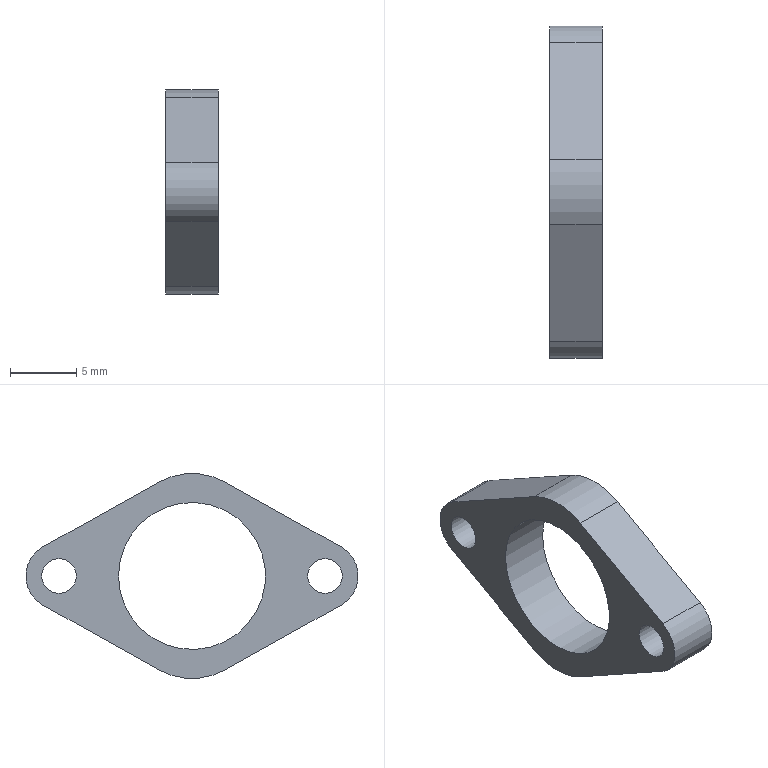Part | STEP file | Dodanie-wyci_gni_cie1_6 | 1 solid | 13 faces | box 3.95 x 25 x 15.427 mm | volume 542.296 mm3 | cylinder 7 | plane 6 | commonest cylinder face diameters 2.6 x2 5 x2 10 x2 11.05 x1
STEP:
#1=CARTESIAN_POINT('',(0.,0.,0.));
#2=DIRECTION('',(0.,0.,1.));
#3=DIRECTION('',(1.,0.,0.));
#4=AXIS2_PLACEMENT_3D('',#1,#2,#3);
#5=CARTESIAN_POINT('',(-64.621,79.561,-75.356));
#6=VERTEX_POINT('',#5);
#7=CARTESIAN_POINT('',(-64.621,78.261,-75.356));
#8=DIRECTION('',(1.,0.,0.));
#9=DIRECTION('',(0.,1.,0.));
#10=AXIS2_PLACEMENT_3D('',#7,#8,#9);
#11=CIRCLE('',#10,1.3);
#12=CARTESIAN_POINT('',(-64.621,78.261,-75.356));
#13=DIRECTION('',(1.,0.,0.));
#14=DIRECTION('',(0.,1.,0.));
#15=AXIS2_PLACEMENT_3D('',#12,#13,#14);
#16=CYLINDRICAL_SURFACE('',#15,1.3);
#17=CARTESIAN_POINT('',(0.,0.));
#18=DIRECTION('',(1.,0.));
#19=VECTOR('',#18,1.);
#20=LINE('',#17,#19);
#21=(GEOMETRIC_REPRESENTATION_CONTEXT(2)PARAMETRIC_REPRESENTATION_CONTEXT()REPRESENTATION_CONTEXT('',''));
#22=DEFINITIONAL_REPRESENTATION('',(#20),#21);
#23=PCURVE('',#16,#22);
#24=CARTESIAN_POINT('',(-64.621,88.261,-75.356));
#25=DIRECTION('',(-1.,0.,0.));
#26=DIRECTION('',(0.,-1.,0.));
#27=AXIS2_PLACEMENT_3D('',#24,#25,#26);
#28=PLANE('',#27);
#29=CARTESIAN_POINT('',(8.7,0.000278));
#30=CARTESIAN_POINT('',(8.7,2.252));
#31=CARTESIAN_POINT('',(10.65,1.126));
#32=CARTESIAN_POINT('',(12.6,0.000278));
#33=CARTESIAN_POINT('',(10.65,-1.126));
#34=CARTESIAN_POINT('',(8.7,-2.251));
#35=CARTESIAN_POINT('',(8.7,0.000278));
#36=(BOUNDED_CURVE()B_SPLINE_CURVE(2,(#29,#30,#31,#32,#33,#34,#35),.UNSPECIFIED.,.T.,.F.)B_SPLINE_CURVE_WITH_KNOTS((1,2,2,2,2,1),(-2.094,0.,2.094,4.189,6.283,8.378),.UNSPECIFIED.)CURVE()GEOMETRIC_REPRESENTATION_ITEM()RATIONAL_B_SPLINE_CURVE((1.,0.5,1.,0.5,1.,0.5,1.))REPRESENTATION_ITEM(''));
#37=(GEOMETRIC_REPRESENTATION_CONTEXT(2)PARAMETRIC_REPRESENTATION_CONTEXT()REPRESENTATION_CONTEXT('',''));
#38=DEFINITIONAL_REPRESENTATION('',(#36),#37);
#39=PCURVE('',#28,#38);
#40=SURFACE_CURVE('',#11,(#23,#39),.PCURVE_S1.);
#41=EDGE_CURVE('',#6,#6,#40,.T.);
#42=ORIENTED_EDGE('',*,*,#41,.T.);
#43=CARTESIAN_POINT('',(-60.671,79.561,-75.356));
#44=VERTEX_POINT('',#43);
#45=CARTESIAN_POINT('',(-60.671,79.561,-75.356));
#46=DIRECTION('',(-1.,0.,0.));
#47=VECTOR('',#46,1.);
#48=LINE('',#45,#47);
#49=CARTESIAN_POINT('',(6.283,3.95));
#50=DIRECTION('',(0.,-1.));
#51=VECTOR('',#50,1.);
#52=LINE('',#49,#51);
#53=(GEOMETRIC_REPRESENTATION_CONTEXT(2)PARAMETRIC_REPRESENTATION_CONTEXT()REPRESENTATION_CONTEXT('',''));
#54=DEFINITIONAL_REPRESENTATION('',(#52),#53);
#55=PCURVE('',#16,#54);
#56=CARTESIAN_POINT('',(0.,3.95));
#57=DIRECTION('',(0.,-1.));
#58=VECTOR('',#57,1.);
#59=LINE('',#56,#58);
#60=(GEOMETRIC_REPRESENTATION_CONTEXT(2)PARAMETRIC_REPRESENTATION_CONTEXT()REPRESENTATION_CONTEXT('',''));
#61=DEFINITIONAL_REPRESENTATION('',(#59),#60);
#62=PCURVE('',#16,#61);
#63=SEAM_CURVE('',#48,(#55,#62),.PCURVE_S1.);
#64=EDGE_CURVE('',#44,#6,#63,.T.);
#65=ORIENTED_EDGE('',*,*,#64,.F.);
#66=CARTESIAN_POINT('',(-60.671,78.261,-75.356));
#67=DIRECTION('',(-1.,0.,0.));
#68=DIRECTION('',(0.,1.,0.));
#69=AXIS2_PLACEMENT_3D('',#66,#67,#68);
#70=CIRCLE('',#69,1.3);
#71=CARTESIAN_POINT('',(6.283,3.95));
#72=DIRECTION('',(-1.,0.));
#73=VECTOR('',#72,1.);
#74=LINE('',#71,#73);
#75=(GEOMETRIC_REPRESENTATION_CONTEXT(2)PARAMETRIC_REPRESENTATION_CONTEXT()REPRESENTATION_CONTEXT('',''));
#76=DEFINITIONAL_REPRESENTATION('',(#74),#75);
#77=PCURVE('',#16,#76);
#78=CARTESIAN_POINT('',(-60.671,88.261,-75.356));
#79=DIRECTION('',(-1.,0.,0.));
#80=DIRECTION('',(0.,-1.,0.));
#81=AXIS2_PLACEMENT_3D('',#78,#79,#80);
#82=PLANE('',#81);
#83=CARTESIAN_POINT('',(10.,0.000278));
#84=DIRECTION('',(-1.,0.));
#85=AXIS2_PLACEMENT_2D('',#83,#84);
#86=CIRCLE('',#85,1.3);
#87=(GEOMETRIC_REPRESENTATION_CONTEXT(2)PARAMETRIC_REPRESENTATION_CONTEXT()REPRESENTATION_CONTEXT('',''));
#88=DEFINITIONAL_REPRESENTATION('',(#86),#87);
#89=PCURVE('',#82,#88);
#90=SURFACE_CURVE('',#70,(#77,#89),.PCURVE_S1.);
#91=EDGE_CURVE('',#44,#44,#90,.T.);
#92=ORIENTED_EDGE('',*,*,#91,.T.);
#93=ORIENTED_EDGE('',*,*,#64,.T.);
#94=EDGE_LOOP('',(#42,#65,#92,#93));
#95=FACE_BOUND('',#94,.F.);
#96=ADVANCED_FACE('',(#95),#16,.F.);
#97=CARTESIAN_POINT('',(-64.621,93.786,-75.356));
#98=VERTEX_POINT('',#97);
#99=CARTESIAN_POINT('',(-64.621,88.261,-75.356));
#100=DIRECTION('',(1.,0.,0.));
#101=DIRECTION('',(0.,1.,0.));
#102=AXIS2_PLACEMENT_3D('',#99,#100,#101);
#103=CIRCLE('',#102,5.525);
#104=CARTESIAN_POINT('',(-64.621,88.261,-75.356));
#105=DIRECTION('',(1.,0.,0.));
#106=DIRECTION('',(0.,1.,0.));
#107=AXIS2_PLACEMENT_3D('',#104,#105,#106);
#108=CYLINDRICAL_SURFACE('',#107,5.525);
#109=CARTESIAN_POINT('',(0.,0.));
#110=DIRECTION('',(1.,0.));
#111=VECTOR('',#110,1.);
#112=LINE('',#109,#111);
#113=(GEOMETRIC_REPRESENTATION_CONTEXT(2)PARAMETRIC_REPRESENTATION_CONTEXT()REPRESENTATION_CONTEXT('',''));
#114=DEFINITIONAL_REPRESENTATION('',(#112),#113);
#115=PCURVE('',#108,#114);
#116=CARTESIAN_POINT('',(-5.525,0.000278));
#117=CARTESIAN_POINT('',(-5.525,9.57));
#118=CARTESIAN_POINT('',(2.763,4.785));
#119=CARTESIAN_POINT('',(11.05,0.000278));
#120=CARTESIAN_POINT('',(2.763,-4.785));
#121=CARTESIAN_POINT('',(-5.525,-9.569));
#122=CARTESIAN_POINT('',(-5.525,0.000278));
#123=(BOUNDED_CURVE()B_SPLINE_CURVE(2,(#116,#117,#118,#119,#120,#121,#122),.UNSPECIFIED.,.T.,.F.)B_SPLINE_CURVE_WITH_KNOTS((1,2,2,2,2,1),(-2.094,0.,2.094,4.189,6.283,8.378),.UNSPECIFIED.)CURVE()GEOMETRIC_REPRESENTATION_ITEM()RATIONAL_B_SPLINE_CURVE((1.,0.5,1.,0.5,1.,0.5,1.))REPRESENTATION_ITEM(''));
#124=(GEOMETRIC_REPRESENTATION_CONTEXT(2)PARAMETRIC_REPRESENTATION_CONTEXT()REPRESENTATION_CONTEXT('',''));
#125=DEFINITIONAL_REPRESENTATION('',(#123),#124);
#126=PCURVE('',#28,#125);
#127=SURFACE_CURVE('',#103,(#115,#126),.PCURVE_S1.);
#128=EDGE_CURVE('',#98,#98,#127,.T.);
#129=ORIENTED_EDGE('',*,*,#128,.T.);
#130=CARTESIAN_POINT('',(-60.671,93.786,-75.356));
#131=VERTEX_POINT('',#130);
#132=CARTESIAN_POINT('',(-60.671,93.786,-75.356));
#133=DIRECTION('',(-1.,0.,0.));
#134=VECTOR('',#133,1.);
#135=LINE('',#132,#134);
#136=CARTESIAN_POINT('',(6.283,3.95));
#137=DIRECTION('',(0.,-1.));
#138=VECTOR('',#137,1.);
#139=LINE('',#136,#138);
#140=(GEOMETRIC_REPRESENTATION_CONTEXT(2)PARAMETRIC_REPRESENTATION_CONTEXT()REPRESENTATION_CONTEXT('',''));
#141=DEFINITIONAL_REPRESENTATION('',(#139),#140);
#142=PCURVE('',#108,#141);
#143=CARTESIAN_POINT('',(0.,3.95));
#144=DIRECTION('',(0.,-1.));
#145=VECTOR('',#144,1.);
#146=LINE('',#143,#145);
#147=(GEOMETRIC_REPRESENTATION_CONTEXT(2)PARAMETRIC_REPRESENTATION_CONTEXT()REPRESENTATION_CONTEXT('',''));
#148=DEFINITIONAL_REPRESENTATION('',(#146),#147);
#149=PCURVE('',#108,#148);
#150=SEAM_CURVE('',#135,(#142,#149),.PCURVE_S1.);
#151=EDGE_CURVE('',#131,#98,#150,.T.);
#152=ORIENTED_EDGE('',*,*,#151,.F.);
#153=CARTESIAN_POINT('',(-60.671,88.261,-75.356));
#154=DIRECTION('',(-1.,0.,0.));
#155=DIRECTION('',(0.,1.,0.));
#156=AXIS2_PLACEMENT_3D('',#153,#154,#155);
#157=CIRCLE('',#156,5.525);
#158=CARTESIAN_POINT('',(6.283,3.95));
#159=DIRECTION('',(-1.,0.));
#160=VECTOR('',#159,1.);
#161=LINE('',#158,#160);
#162=(GEOMETRIC_REPRESENTATION_CONTEXT(2)PARAMETRIC_REPRESENTATION_CONTEXT()REPRESENTATION_CONTEXT('',''));
#163=DEFINITIONAL_REPRESENTATION('',(#161),#162);
#164=PCURVE('',#108,#163);
#165=CARTESIAN_POINT('',(0.,0.000278));
#166=DIRECTION('',(-1.,0.));
#167=AXIS2_PLACEMENT_2D('',#165,#166);
#168=CIRCLE('',#167,5.525);
#169=(GEOMETRIC_REPRESENTATION_CONTEXT(2)PARAMETRIC_REPRESENTATION_CONTEXT()REPRESENTATION_CONTEXT('',''));
#170=DEFINITIONAL_REPRESENTATION('',(#168),#169);
#171=PCURVE('',#82,#170);
#172=SURFACE_CURVE('',#157,(#164,#171),.PCURVE_S1.);
#173=EDGE_CURVE('',#131,#131,#172,.T.);
#174=ORIENTED_EDGE('',*,*,#173,.T.);
#175=ORIENTED_EDGE('',*,*,#151,.T.);
#176=EDGE_LOOP('',(#129,#152,#174,#175));
#177=FACE_BOUND('',#176,.F.);
#178=ADVANCED_FACE('',(#177),#108,.F.);
#179=CARTESIAN_POINT('',(-64.621,99.561,-75.356));
#180=VERTEX_POINT('',#179);
#181=CARTESIAN_POINT('',(-64.621,98.261,-75.356));
#182=DIRECTION('',(1.,0.,0.));
#183=DIRECTION('',(0.,1.,0.));
#184=AXIS2_PLACEMENT_3D('',#181,#182,#183);
#185=CIRCLE('',#184,1.3);
#186=CARTESIAN_POINT('',(-64.621,98.261,-75.356));
#187=DIRECTION('',(1.,0.,0.));
#188=DIRECTION('',(0.,1.,0.));
#189=AXIS2_PLACEMENT_3D('',#186,#187,#188);
#190=CYLINDRICAL_SURFACE('',#189,1.3);
#191=CARTESIAN_POINT('',(0.,0.));
#192=DIRECTION('',(1.,0.));
#193=VECTOR('',#192,1.);
#194=LINE('',#191,#193);
#195=(GEOMETRIC_REPRESENTATION_CONTEXT(2)PARAMETRIC_REPRESENTATION_CONTEXT()REPRESENTATION_CONTEXT('',''));
#196=DEFINITIONAL_REPRESENTATION('',(#194),#195);
#197=PCURVE('',#190,#196);
#198=CARTESIAN_POINT('',(-11.3,0.000278));
#199=CARTESIAN_POINT('',(-11.3,2.252));
#200=CARTESIAN_POINT('',(-9.35,1.126));
#201=CARTESIAN_POINT('',(-7.4,0.000278));
#202=CARTESIAN_POINT('',(-9.35,-1.126));
#203=CARTESIAN_POINT('',(-11.3,-2.251));
#204=CARTESIAN_POINT('',(-11.3,0.000278));
#205=(BOUNDED_CURVE()B_SPLINE_CURVE(2,(#198,#199,#200,#201,#202,#203,#204),.UNSPECIFIED.,.T.,.F.)B_SPLINE_CURVE_WITH_KNOTS((1,2,2,2,2,1),(-2.094,0.,2.094,4.189,6.283,8.378),.UNSPECIFIED.)CURVE()GEOMETRIC_REPRESENTATION_ITEM()RATIONAL_B_SPLINE_CURVE((1.,0.5,1.,0.5,1.,0.5,1.))REPRESENTATION_ITEM(''));
#206=(GEOMETRIC_REPRESENTATION_CONTEXT(2)PARAMETRIC_REPRESENTATION_CONTEXT()REPRESENTATION_CONTEXT('',''));
#207=DEFINITIONAL_REPRESENTATION('',(#205),#206);
#208=PCURVE('',#28,#207);
#209=SURFACE_CURVE('',#185,(#197,#208),.PCURVE_S1.);
#210=EDGE_CURVE('',#180,#180,#209,.T.);
#211=ORIENTED_EDGE('',*,*,#210,.T.);
#212=CARTESIAN_POINT('',(-60.671,99.561,-75.356));
#213=VERTEX_POINT('',#212);
#214=CARTESIAN_POINT('',(-60.671,99.561,-75.356));
#215=DIRECTION('',(-1.,0.,0.));
#216=VECTOR('',#215,1.);
#217=LINE('',#214,#216);
#218=CARTESIAN_POINT('',(6.283,3.95));
#219=DIRECTION('',(0.,-1.));
#220=VECTOR('',#219,1.);
#221=LINE('',#218,#220);
#222=(GEOMETRIC_REPRESENTATION_CONTEXT(2)PARAMETRIC_REPRESENTATION_CONTEXT()REPRESENTATION_CONTEXT('',''));
#223=DEFINITIONAL_REPRESENTATION('',(#221),#222);
#224=PCURVE('',#190,#223);
#225=CARTESIAN_POINT('',(0.,3.95));
#226=DIRECTION('',(0.,-1.));
#227=VECTOR('',#226,1.);
#228=LINE('',#225,#227);
#229=(GEOMETRIC_REPRESENTATION_CONTEXT(2)PARAMETRIC_REPRESENTATION_CONTEXT()REPRESENTATION_CONTEXT('',''));
#230=DEFINITIONAL_REPRESENTATION('',(#228),#229);
#231=PCURVE('',#190,#230);
#232=SEAM_CURVE('',#217,(#224,#231),.PCURVE_S1.);
#233=EDGE_CURVE('',#213,#180,#232,.T.);
#234=ORIENTED_EDGE('',*,*,#233,.F.);
#235=CARTESIAN_POINT('',(-60.671,98.261,-75.356));
#236=DIRECTION('',(-1.,0.,0.));
#237=DIRECTION('',(0.,1.,0.));
#238=AXIS2_PLACEMENT_3D('',#235,#236,#237);
#239=CIRCLE('',#238,1.3);
#240=CARTESIAN_POINT('',(6.283,3.95));
#241=DIRECTION('',(-1.,0.));
#242=VECTOR('',#241,1.);
#243=LINE('',#240,#242);
#244=(GEOMETRIC_REPRESENTATION_CONTEXT(2)PARAMETRIC_REPRESENTATION_CONTEXT()REPRESENTATION_CONTEXT('',''));
#245=DEFINITIONAL_REPRESENTATION('',(#243),#244);
#246=PCURVE('',#190,#245);
#247=CARTESIAN_POINT('',(-10.,0.000278));
#248=DIRECTION('',(-1.,0.));
#249=AXIS2_PLACEMENT_2D('',#247,#248);
#250=CIRCLE('',#249,1.3);
#251=(GEOMETRIC_REPRESENTATION_CONTEXT(2)PARAMETRIC_REPRESENTATION_CONTEXT()REPRESENTATION_CONTEXT('',''));
#252=DEFINITIONAL_REPRESENTATION('',(#250),#251);
#253=PCURVE('',#82,#252);
#254=SURFACE_CURVE('',#239,(#246,#253),.PCURVE_S1.);
#255=EDGE_CURVE('',#213,#213,#254,.T.);
#256=ORIENTED_EDGE('',*,*,#255,.T.);
#257=ORIENTED_EDGE('',*,*,#233,.T.);
#258=EDGE_LOOP('',(#211,#234,#256,#257));
#259=FACE_BOUND('',#258,.F.);
#260=ADVANCED_FACE('',(#259),#190,.F.);
#261=ORIENTED_EDGE('',*,*,#41,.T.);
#262=EDGE_LOOP('',(#261));
#263=FACE_BOUND('',#262,.T.);
#264=ORIENTED_EDGE('',*,*,#128,.T.);
#265=EDGE_LOOP('',(#264));
#266=FACE_BOUND('',#265,.T.);
#267=ORIENTED_EDGE('',*,*,#210,.T.);
#268=EDGE_LOOP('',(#267));
#269=FACE_BOUND('',#268,.T.);
#270=CARTESIAN_POINT('',(-64.621,85.826,-68.276));
#271=VERTEX_POINT('',#270);
#272=CARTESIAN_POINT('',(-64.621,90.696,-68.276));
#273=VERTEX_POINT('',#272);
#274=CARTESIAN_POINT('',(-64.621,88.261,-72.643));
#275=DIRECTION('',(-1.,0.,0.));
#276=DIRECTION('',(0.,1.,0.));
#277=AXIS2_PLACEMENT_3D('',#274,#275,#276);
#278=CIRCLE('',#277,5.);
#279=CARTESIAN_POINT('',(0.,2.713));
#280=DIRECTION('',(-1.,0.));
#281=AXIS2_PLACEMENT_2D('',#279,#280);
#282=CIRCLE('',#281,5.);
#283=(GEOMETRIC_REPRESENTATION_CONTEXT(2)PARAMETRIC_REPRESENTATION_CONTEXT()REPRESENTATION_CONTEXT('',''));
#284=DEFINITIONAL_REPRESENTATION('',(#282),#283);
#285=PCURVE('',#28,#284);
#286=CARTESIAN_POINT('',(-64.621,88.261,-72.643));
#287=DIRECTION('',(1.,0.,0.));
#288=DIRECTION('',(0.,1.,0.));
#289=AXIS2_PLACEMENT_3D('',#286,#287,#288);
#290=CYLINDRICAL_SURFACE('',#289,5.);
#291=CARTESIAN_POINT('',(6.283,0.));
#292=DIRECTION('',(-1.,0.));
#293=VECTOR('',#292,1.);
#294=LINE('',#291,#293);
#295=(GEOMETRIC_REPRESENTATION_CONTEXT(2)PARAMETRIC_REPRESENTATION_CONTEXT()REPRESENTATION_CONTEXT('',''));
#296=DEFINITIONAL_REPRESENTATION('',(#294),#295);
#297=PCURVE('',#290,#296);
#298=SURFACE_CURVE('',#278,(#285,#297),.PCURVE_S1.);
#299=EDGE_CURVE('',#271,#273,#298,.T.);
#300=ORIENTED_EDGE('',*,*,#299,.T.);
#301=CARTESIAN_POINT('',(-64.621,99.478,-73.172));
#302=VERTEX_POINT('',#301);
#303=CARTESIAN_POINT('',(-64.621,90.696,-68.276));
#304=DIRECTION('',(0.,0.8734,-0.487));
#305=VECTOR('',#304,1.);
#306=LINE('',#303,#305);
#307=CARTESIAN_POINT('',(-2.435,7.08));
#308=DIRECTION('',(-0.8734,-0.487));
#309=VECTOR('',#308,1.);
#310=LINE('',#307,#309);
#311=(GEOMETRIC_REPRESENTATION_CONTEXT(2)PARAMETRIC_REPRESENTATION_CONTEXT()REPRESENTATION_CONTEXT('',''));
#312=DEFINITIONAL_REPRESENTATION('',(#310),#311);
#313=PCURVE('',#28,#312);
#314=CARTESIAN_POINT('',(-62.646,95.087,-70.724));
#315=DIRECTION('',(0.,-0.487,-0.8734));
#316=DIRECTION('',(0.,-0.8734,0.487));
#317=AXIS2_PLACEMENT_3D('',#314,#315,#316);
#318=PLANE('',#317);
#319=CARTESIAN_POINT('',(5.028,1.975));
#320=DIRECTION('',(-1.,0.));
#321=VECTOR('',#320,1.);
#322=LINE('',#319,#321);
#323=(GEOMETRIC_REPRESENTATION_CONTEXT(2)PARAMETRIC_REPRESENTATION_CONTEXT()REPRESENTATION_CONTEXT('',''));
#324=DEFINITIONAL_REPRESENTATION('',(#322),#323);
#325=PCURVE('',#318,#324);
#326=SURFACE_CURVE('',#306,(#313,#325),.PCURVE_S1.);
#327=EDGE_CURVE('',#273,#302,#326,.T.);
#328=ORIENTED_EDGE('',*,*,#327,.T.);
#329=CARTESIAN_POINT('',(-64.621,99.478,-77.539));
#330=VERTEX_POINT('',#329);
#331=CARTESIAN_POINT('',(-64.621,98.261,-75.356));
#332=DIRECTION('',(-1.,0.,0.));
#333=DIRECTION('',(0.,0.,1.));
#334=AXIS2_PLACEMENT_3D('',#331,#332,#333);
#335=CIRCLE('',#334,2.5);
#336=CARTESIAN_POINT('',(-10.,0.000278));
#337=DIRECTION('',(0.,1.));
#338=AXIS2_PLACEMENT_2D('',#336,#337);
#339=CIRCLE('',#338,2.5);
#340=(GEOMETRIC_REPRESENTATION_CONTEXT(2)PARAMETRIC_REPRESENTATION_CONTEXT()REPRESENTATION_CONTEXT('',''));
#341=DEFINITIONAL_REPRESENTATION('',(#339),#340);
#342=PCURVE('',#28,#341);
#343=CARTESIAN_POINT('',(-64.621,98.261,-75.356));
#344=DIRECTION('',(1.,0.,0.));
#345=DIRECTION('',(0.,0.,1.));
#346=AXIS2_PLACEMENT_3D('',#343,#344,#345);
#347=CYLINDRICAL_SURFACE('',#346,2.5);
#348=CARTESIAN_POINT('',(6.283,0.));
#349=DIRECTION('',(-1.,0.));
#350=VECTOR('',#349,1.);
#351=LINE('',#348,#350);
#352=(GEOMETRIC_REPRESENTATION_CONTEXT(2)PARAMETRIC_REPRESENTATION_CONTEXT()REPRESENTATION_CONTEXT('',''));
#353=DEFINITIONAL_REPRESENTATION('',(#351),#352);
#354=PCURVE('',#347,#353);
#355=SURFACE_CURVE('',#335,(#342,#354),.PCURVE_S1.);
#356=EDGE_CURVE('',#302,#330,#355,.T.);
#357=ORIENTED_EDGE('',*,*,#356,.T.);
#358=CARTESIAN_POINT('',(-64.621,90.696,-82.436));
#359=VERTEX_POINT('',#358);
#360=CARTESIAN_POINT('',(-64.621,99.478,-77.539));
#361=DIRECTION('',(0.,-0.8734,-0.487));
#362=VECTOR('',#361,1.);
#363=LINE('',#360,#362);
#364=CARTESIAN_POINT('',(-11.218,-2.183));
#365=DIRECTION('',(0.8734,-0.487));
#366=VECTOR('',#365,1.);
#367=LINE('',#364,#366);
#368=(GEOMETRIC_REPRESENTATION_CONTEXT(2)PARAMETRIC_REPRESENTATION_CONTEXT()REPRESENTATION_CONTEXT('',''));
#369=DEFINITIONAL_REPRESENTATION('',(#367),#368);
#370=PCURVE('',#28,#369);
#371=CARTESIAN_POINT('',(-62.646,95.087,-79.988));
#372=DIRECTION('',(0.,-0.487,0.8734));
#373=DIRECTION('',(0.,0.8734,0.487));
#374=AXIS2_PLACEMENT_3D('',#371,#372,#373);
#375=PLANE('',#374);
#376=CARTESIAN_POINT('',(5.028,1.975));
#377=DIRECTION('',(-1.,0.));
#378=VECTOR('',#377,1.);
#379=LINE('',#376,#378);
#380=(GEOMETRIC_REPRESENTATION_CONTEXT(2)PARAMETRIC_REPRESENTATION_CONTEXT()REPRESENTATION_CONTEXT('',''));
#381=DEFINITIONAL_REPRESENTATION('',(#379),#380);
#382=PCURVE('',#375,#381);
#383=SURFACE_CURVE('',#363,(#370,#382),.PCURVE_S1.);
#384=EDGE_CURVE('',#330,#359,#383,.T.);
#385=ORIENTED_EDGE('',*,*,#384,.T.);
#386=CARTESIAN_POINT('',(-64.621,85.826,-82.436));
#387=VERTEX_POINT('',#386);
#388=CARTESIAN_POINT('',(-64.621,88.261,-78.069));
#389=DIRECTION('',(-1.,0.,0.));
#390=DIRECTION('',(0.,1.,0.));
#391=AXIS2_PLACEMENT_3D('',#388,#389,#390);
#392=CIRCLE('',#391,5.);
#393=CARTESIAN_POINT('',(0.,-2.713));
#394=DIRECTION('',(-1.,0.));
#395=AXIS2_PLACEMENT_2D('',#393,#394);
#396=CIRCLE('',#395,5.);
#397=(GEOMETRIC_REPRESENTATION_CONTEXT(2)PARAMETRIC_REPRESENTATION_CONTEXT()REPRESENTATION_CONTEXT('',''));
#398=DEFINITIONAL_REPRESENTATION('',(#396),#397);
#399=PCURVE('',#28,#398);
#400=CARTESIAN_POINT('',(-64.621,88.261,-78.069));
#401=DIRECTION('',(1.,0.,0.));
#402=DIRECTION('',(0.,1.,0.));
#403=AXIS2_PLACEMENT_3D('',#400,#401,#402);
#404=CYLINDRICAL_SURFACE('',#403,5.);
#405=CARTESIAN_POINT('',(6.283,0.));
#406=DIRECTION('',(-1.,0.));
#407=VECTOR('',#406,1.);
#408=LINE('',#405,#407);
#409=(GEOMETRIC_REPRESENTATION_CONTEXT(2)PARAMETRIC_REPRESENTATION_CONTEXT()REPRESENTATION_CONTEXT('',''));
#410=DEFINITIONAL_REPRESENTATION('',(#408),#409);
#411=PCURVE('',#404,#410);
#412=SURFACE_CURVE('',#392,(#399,#411),.PCURVE_S1.);
#413=EDGE_CURVE('',#359,#387,#412,.T.);
#414=ORIENTED_EDGE('',*,*,#413,.T.);
#415=CARTESIAN_POINT('',(-64.621,77.043,-77.539));
#416=VERTEX_POINT('',#415);
#417=CARTESIAN_POINT('',(-64.621,85.826,-82.436));
#418=DIRECTION('',(0.,-0.8734,0.487));
#419=VECTOR('',#418,1.);
#420=LINE('',#417,#419);
#421=CARTESIAN_POINT('',(2.435,-7.08));
#422=DIRECTION('',(0.8734,0.487));
#423=VECTOR('',#422,1.);
#424=LINE('',#421,#423);
#425=(GEOMETRIC_REPRESENTATION_CONTEXT(2)PARAMETRIC_REPRESENTATION_CONTEXT()REPRESENTATION_CONTEXT('',''));
#426=DEFINITIONAL_REPRESENTATION('',(#424),#425);
#427=PCURVE('',#28,#426);
#428=CARTESIAN_POINT('',(-62.646,81.435,-79.988));
#429=DIRECTION('',(0.,0.487,0.8734));
#430=DIRECTION('',(0.,0.8734,-0.487));
#431=AXIS2_PLACEMENT_3D('',#428,#429,#430);
#432=PLANE('',#431);
#433=CARTESIAN_POINT('',(5.028,1.975));
#434=DIRECTION('',(-1.,0.));
#435=VECTOR('',#434,1.);
#436=LINE('',#433,#435);
#437=(GEOMETRIC_REPRESENTATION_CONTEXT(2)PARAMETRIC_REPRESENTATION_CONTEXT()REPRESENTATION_CONTEXT('',''));
#438=DEFINITIONAL_REPRESENTATION('',(#436),#437);
#439=PCURVE('',#432,#438);
#440=SURFACE_CURVE('',#420,(#427,#439),.PCURVE_S1.);
#441=EDGE_CURVE('',#387,#416,#440,.T.);
#442=ORIENTED_EDGE('',*,*,#441,.T.);
#443=CARTESIAN_POINT('',(-64.621,77.043,-73.172));
#444=VERTEX_POINT('',#443);
#445=CARTESIAN_POINT('',(-64.621,78.261,-75.356));
#446=DIRECTION('',(-1.,0.,0.));
#447=DIRECTION('',(0.,0.,1.));
#448=AXIS2_PLACEMENT_3D('',#445,#446,#447);
#449=CIRCLE('',#448,2.5);
#450=CARTESIAN_POINT('',(10.,0.000278));
#451=DIRECTION('',(0.,1.));
#452=AXIS2_PLACEMENT_2D('',#450,#451);
#453=CIRCLE('',#452,2.5);
#454=(GEOMETRIC_REPRESENTATION_CONTEXT(2)PARAMETRIC_REPRESENTATION_CONTEXT()REPRESENTATION_CONTEXT('',''));
#455=DEFINITIONAL_REPRESENTATION('',(#453),#454);
#456=PCURVE('',#28,#455);
#457=CARTESIAN_POINT('',(-64.621,78.261,-75.356));
#458=DIRECTION('',(1.,0.,0.));
#459=DIRECTION('',(0.,0.,1.));
#460=AXIS2_PLACEMENT_3D('',#457,#458,#459);
#461=CYLINDRICAL_SURFACE('',#460,2.5);
#462=CARTESIAN_POINT('',(6.283,0.));
#463=DIRECTION('',(-1.,0.));
#464=VECTOR('',#463,1.);
#465=LINE('',#462,#464);
#466=(GEOMETRIC_REPRESENTATION_CONTEXT(2)PARAMETRIC_REPRESENTATION_CONTEXT()REPRESENTATION_CONTEXT('',''));
#467=DEFINITIONAL_REPRESENTATION('',(#465),#466);
#468=PCURVE('',#461,#467);
#469=SURFACE_CURVE('',#449,(#456,#468),.PCURVE_S1.);
#470=EDGE_CURVE('',#416,#444,#469,.T.);
#471=ORIENTED_EDGE('',*,*,#470,.T.);
#472=CARTESIAN_POINT('',(-64.621,77.043,-73.172));
#473=DIRECTION('',(0.,0.8734,0.487));
#474=VECTOR('',#473,1.);
#475=LINE('',#472,#474);
#476=CARTESIAN_POINT('',(11.217,2.184));
#477=DIRECTION('',(-0.8734,0.487));
#478=VECTOR('',#477,1.);
#479=LINE('',#476,#478);
#480=(GEOMETRIC_REPRESENTATION_CONTEXT(2)PARAMETRIC_REPRESENTATION_CONTEXT()REPRESENTATION_CONTEXT('',''));
#481=DEFINITIONAL_REPRESENTATION('',(#479),#480);
#482=PCURVE('',#28,#481);
#483=CARTESIAN_POINT('',(-62.646,81.435,-70.724));
#484=DIRECTION('',(0.,0.487,-0.8734));
#485=DIRECTION('',(0.,-0.8734,-0.487));
#486=AXIS2_PLACEMENT_3D('',#483,#484,#485);
#487=PLANE('',#486);
#488=CARTESIAN_POINT('',(5.028,1.975));
#489=DIRECTION('',(-1.,0.));
#490=VECTOR('',#489,1.);
#491=LINE('',#488,#490);
#492=(GEOMETRIC_REPRESENTATION_CONTEXT(2)PARAMETRIC_REPRESENTATION_CONTEXT()REPRESENTATION_CONTEXT('',''));
#493=DEFINITIONAL_REPRESENTATION('',(#491),#492);
#494=PCURVE('',#487,#493);
#495=SURFACE_CURVE('',#475,(#482,#494),.PCURVE_S1.);
#496=EDGE_CURVE('',#444,#271,#495,.T.);
#497=ORIENTED_EDGE('',*,*,#496,.T.);
#498=EDGE_LOOP('',(#300,#328,#357,#385,#414,#442,#471,#497));
#499=FACE_BOUND('',#498,.T.);
#500=ADVANCED_FACE('',(#263,#266,#269,#499),#28,.T.);
#501=CARTESIAN_POINT('',(-60.671,99.478,-73.172));
#502=VERTEX_POINT('',#501);
#503=CARTESIAN_POINT('',(-64.621,99.478,-73.172));
#504=DIRECTION('',(1.,0.,0.));
#505=VECTOR('',#504,1.);
#506=LINE('',#503,#505);
#507=CARTESIAN_POINT('',(-5.028,1.975));
#508=DIRECTION('',(0.,-1.));
#509=VECTOR('',#508,1.);
#510=LINE('',#507,#509);
#511=(GEOMETRIC_REPRESENTATION_CONTEXT(2)PARAMETRIC_REPRESENTATION_CONTEXT()REPRESENTATION_CONTEXT('',''));
#512=DEFINITIONAL_REPRESENTATION('',(#510),#511);
#513=PCURVE('',#318,#512);
#514=CARTESIAN_POINT('',(5.775,0.));
#515=DIRECTION('',(0.,1.));
#516=VECTOR('',#515,1.);
#517=LINE('',#514,#516);
#518=(GEOMETRIC_REPRESENTATION_CONTEXT(2)PARAMETRIC_REPRESENTATION_CONTEXT()REPRESENTATION_CONTEXT('',''));
#519=DEFINITIONAL_REPRESENTATION('',(#517),#518);
#520=PCURVE('',#347,#519);
#521=SURFACE_CURVE('',#506,(#513,#520),.PCURVE_S1.);
#522=EDGE_CURVE('',#302,#502,#521,.T.);
#523=ORIENTED_EDGE('',*,*,#522,.F.);
#524=ORIENTED_EDGE('',*,*,#327,.F.);
#525=CARTESIAN_POINT('',(-60.671,90.696,-68.276));
#526=VERTEX_POINT('',#525);
#527=CARTESIAN_POINT('',(-60.671,90.696,-68.276));
#528=DIRECTION('',(-1.,0.,0.));
#529=VECTOR('',#528,1.);
#530=LINE('',#527,#529);
#531=CARTESIAN_POINT('',(5.028,-1.975));
#532=DIRECTION('',(0.,1.));
#533=VECTOR('',#532,1.);
#534=LINE('',#531,#533);
#535=(GEOMETRIC_REPRESENTATION_CONTEXT(2)PARAMETRIC_REPRESENTATION_CONTEXT()REPRESENTATION_CONTEXT('',''));
#536=DEFINITIONAL_REPRESENTATION('',(#534),#535);
#537=PCURVE('',#318,#536);
#538=CARTESIAN_POINT('',(1.062,3.95));
#539=DIRECTION('',(0.,-1.));
#540=VECTOR('',#539,1.);
#541=LINE('',#538,#540);
#542=(GEOMETRIC_REPRESENTATION_CONTEXT(2)PARAMETRIC_REPRESENTATION_CONTEXT()REPRESENTATION_CONTEXT('',''));
#543=DEFINITIONAL_REPRESENTATION('',(#541),#542);
#544=PCURVE('',#290,#543);
#545=SURFACE_CURVE('',#530,(#537,#544),.PCURVE_S1.);
#546=EDGE_CURVE('',#526,#273,#545,.T.);
#547=ORIENTED_EDGE('',*,*,#546,.F.);
#548=CARTESIAN_POINT('',(-60.671,99.478,-73.172));
#549=DIRECTION('',(0.,-0.8734,0.487));
#550=VECTOR('',#549,1.);
#551=LINE('',#548,#550);
#552=CARTESIAN_POINT('',(-5.028,-1.975));
#553=DIRECTION('',(1.,0.));
#554=VECTOR('',#553,1.);
#555=LINE('',#552,#554);
#556=(GEOMETRIC_REPRESENTATION_CONTEXT(2)PARAMETRIC_REPRESENTATION_CONTEXT()REPRESENTATION_CONTEXT('',''));
#557=DEFINITIONAL_REPRESENTATION('',(#555),#556);
#558=PCURVE('',#318,#557);
#559=CARTESIAN_POINT('',(-11.217,2.184));
#560=DIRECTION('',(0.8734,0.487));
#561=VECTOR('',#560,1.);
#562=LINE('',#559,#561);
#563=(GEOMETRIC_REPRESENTATION_CONTEXT(2)PARAMETRIC_REPRESENTATION_CONTEXT()REPRESENTATION_CONTEXT('',''));
#564=DEFINITIONAL_REPRESENTATION('',(#562),#563);
#565=PCURVE('',#82,#564);
#566=SURFACE_CURVE('',#551,(#558,#565),.PCURVE_S1.);
#567=EDGE_CURVE('',#502,#526,#566,.T.);
#568=ORIENTED_EDGE('',*,*,#567,.F.);
#569=EDGE_LOOP('',(#523,#524,#547,#568));
#570=FACE_BOUND('',#569,.T.);
#571=ADVANCED_FACE('',(#570),#318,.F.);
#572=ORIENTED_EDGE('',*,*,#299,.F.);
#573=CARTESIAN_POINT('',(-60.671,85.826,-68.276));
#574=VERTEX_POINT('',#573);
#575=CARTESIAN_POINT('',(-64.621,85.826,-68.276));
#576=DIRECTION('',(1.,0.,0.));
#577=VECTOR('',#576,1.);
#578=LINE('',#575,#577);
#579=CARTESIAN_POINT('',(2.079,0.));
#580=DIRECTION('',(0.,1.));
#581=VECTOR('',#580,1.);
#582=LINE('',#579,#581);
#583=(GEOMETRIC_REPRESENTATION_CONTEXT(2)PARAMETRIC_REPRESENTATION_CONTEXT()REPRESENTATION_CONTEXT('',''));
#584=DEFINITIONAL_REPRESENTATION('',(#582),#583);
#585=PCURVE('',#290,#584);
#586=CARTESIAN_POINT('',(-5.028,1.975));
#587=DIRECTION('',(0.,-1.));
#588=VECTOR('',#587,1.);
#589=LINE('',#586,#588);
#590=(GEOMETRIC_REPRESENTATION_CONTEXT(2)PARAMETRIC_REPRESENTATION_CONTEXT()REPRESENTATION_CONTEXT('',''));
#591=DEFINITIONAL_REPRESENTATION('',(#589),#590);
#592=PCURVE('',#487,#591);
#593=SURFACE_CURVE('',#578,(#585,#592),.PCURVE_S1.);
#594=EDGE_CURVE('',#271,#574,#593,.T.);
#595=ORIENTED_EDGE('',*,*,#594,.T.);
#596=CARTESIAN_POINT('',(-60.671,88.261,-72.643));
#597=DIRECTION('',(-1.,0.,0.));
#598=DIRECTION('',(0.,1.,0.));
#599=AXIS2_PLACEMENT_3D('',#596,#597,#598);
#600=CIRCLE('',#599,5.);
#601=CARTESIAN_POINT('',(6.283,3.95));
#602=DIRECTION('',(-1.,0.));
#603=VECTOR('',#602,1.);
#604=LINE('',#601,#603);
#605=(GEOMETRIC_REPRESENTATION_CONTEXT(2)PARAMETRIC_REPRESENTATION_CONTEXT()REPRESENTATION_CONTEXT('',''));
#606=DEFINITIONAL_REPRESENTATION('',(#604),#605);
#607=PCURVE('',#290,#606);
#608=CARTESIAN_POINT('',(0.,2.713));
#609=DIRECTION('',(-1.,0.));
#610=AXIS2_PLACEMENT_2D('',#608,#609);
#611=CIRCLE('',#610,5.);
#612=(GEOMETRIC_REPRESENTATION_CONTEXT(2)PARAMETRIC_REPRESENTATION_CONTEXT()REPRESENTATION_CONTEXT('',''));
#613=DEFINITIONAL_REPRESENTATION('',(#611),#612);
#614=PCURVE('',#82,#613);
#615=SURFACE_CURVE('',#600,(#607,#614),.PCURVE_S1.);
#616=EDGE_CURVE('',#574,#526,#615,.T.);
#617=ORIENTED_EDGE('',*,*,#616,.T.);
#618=ORIENTED_EDGE('',*,*,#546,.T.);
#619=EDGE_LOOP('',(#572,#595,#617,#618));
#620=FACE_BOUND('',#619,.T.);
#621=ADVANCED_FACE('',(#620),#290,.T.);
#622=ORIENTED_EDGE('',*,*,#594,.F.);
#623=ORIENTED_EDGE('',*,*,#496,.F.);
#624=CARTESIAN_POINT('',(-60.671,77.043,-73.172));
#625=VERTEX_POINT('',#624);
#626=CARTESIAN_POINT('',(-60.671,77.043,-73.172));
#627=DIRECTION('',(-1.,0.,0.));
#628=VECTOR('',#627,1.);
#629=LINE('',#626,#628);
#630=CARTESIAN_POINT('',(5.028,-1.975));
#631=DIRECTION('',(0.,1.));
#632=VECTOR('',#631,1.);
#633=LINE('',#630,#632);
#634=(GEOMETRIC_REPRESENTATION_CONTEXT(2)PARAMETRIC_REPRESENTATION_CONTEXT()REPRESENTATION_CONTEXT('',''));
#635=DEFINITIONAL_REPRESENTATION('',(#633),#634);
#636=PCURVE('',#487,#635);
#637=CARTESIAN_POINT('',(0.5086,3.95));
#638=DIRECTION('',(0.,-1.));
#639=VECTOR('',#638,1.);
#640=LINE('',#637,#639);
#641=(GEOMETRIC_REPRESENTATION_CONTEXT(2)PARAMETRIC_REPRESENTATION_CONTEXT()REPRESENTATION_CONTEXT('',''));
#642=DEFINITIONAL_REPRESENTATION('',(#640),#641);
#643=PCURVE('',#461,#642);
#644=SURFACE_CURVE('',#629,(#636,#643),.PCURVE_S1.);
#645=EDGE_CURVE('',#625,#444,#644,.T.);
#646=ORIENTED_EDGE('',*,*,#645,.F.);
#647=CARTESIAN_POINT('',(-60.671,85.826,-68.276));
#648=DIRECTION('',(0.,-0.8734,-0.487));
#649=VECTOR('',#648,1.);
#650=LINE('',#647,#649);
#651=CARTESIAN_POINT('',(-5.028,-1.975));
#652=DIRECTION('',(1.,0.));
#653=VECTOR('',#652,1.);
#654=LINE('',#651,#653);
#655=(GEOMETRIC_REPRESENTATION_CONTEXT(2)PARAMETRIC_REPRESENTATION_CONTEXT()REPRESENTATION_CONTEXT('',''));
#656=DEFINITIONAL_REPRESENTATION('',(#654),#655);
#657=PCURVE('',#487,#656);
#658=CARTESIAN_POINT('',(2.435,7.08));
#659=DIRECTION('',(0.8734,-0.487));
#660=VECTOR('',#659,1.);
#661=LINE('',#658,#660);
#662=(GEOMETRIC_REPRESENTATION_CONTEXT(2)PARAMETRIC_REPRESENTATION_CONTEXT()REPRESENTATION_CONTEXT('',''));
#663=DEFINITIONAL_REPRESENTATION('',(#661),#662);
#664=PCURVE('',#82,#663);
#665=SURFACE_CURVE('',#650,(#657,#664),.PCURVE_S1.);
#666=EDGE_CURVE('',#574,#625,#665,.T.);
#667=ORIENTED_EDGE('',*,*,#666,.F.);
#668=EDGE_LOOP('',(#622,#623,#646,#667));
#669=FACE_BOUND('',#668,.T.);
#670=ADVANCED_FACE('',(#669),#487,.F.);
#671=ORIENTED_EDGE('',*,*,#470,.F.);
#672=CARTESIAN_POINT('',(-60.671,77.043,-77.539));
#673=VERTEX_POINT('',#672);
#674=CARTESIAN_POINT('',(-64.621,77.043,-77.539));
#675=DIRECTION('',(1.,0.,0.));
#676=VECTOR('',#675,1.);
#677=LINE('',#674,#676);
#678=CARTESIAN_POINT('',(2.633,0.));
#679=DIRECTION('',(0.,1.));
#680=VECTOR('',#679,1.);
#681=LINE('',#678,#680);
#682=(GEOMETRIC_REPRESENTATION_CONTEXT(2)PARAMETRIC_REPRESENTATION_CONTEXT()REPRESENTATION_CONTEXT('',''));
#683=DEFINITIONAL_REPRESENTATION('',(#681),#682);
#684=PCURVE('',#461,#683);
#685=CARTESIAN_POINT('',(-5.028,1.975));
#686=DIRECTION('',(0.,-1.));
#687=VECTOR('',#686,1.);
#688=LINE('',#685,#687);
#689=(GEOMETRIC_REPRESENTATION_CONTEXT(2)PARAMETRIC_REPRESENTATION_CONTEXT()REPRESENTATION_CONTEXT('',''));
#690=DEFINITIONAL_REPRESENTATION('',(#688),#689);
#691=PCURVE('',#432,#690);
#692=SURFACE_CURVE('',#677,(#684,#691),.PCURVE_S1.);
#693=EDGE_CURVE('',#416,#673,#692,.T.);
#694=ORIENTED_EDGE('',*,*,#693,.T.);
#695=CARTESIAN_POINT('',(-60.671,78.261,-75.356));
#696=DIRECTION('',(-1.,0.,0.));
#697=DIRECTION('',(0.,0.,1.));
#698=AXIS2_PLACEMENT_3D('',#695,#696,#697);
#699=CIRCLE('',#698,2.5);
#700=CARTESIAN_POINT('',(6.283,3.95));
#701=DIRECTION('',(-1.,0.));
#702=VECTOR('',#701,1.);
#703=LINE('',#700,#702);
#704=(GEOMETRIC_REPRESENTATION_CONTEXT(2)PARAMETRIC_REPRESENTATION_CONTEXT()REPRESENTATION_CONTEXT('',''));
#705=DEFINITIONAL_REPRESENTATION('',(#703),#704);
#706=PCURVE('',#461,#705);
#707=CARTESIAN_POINT('',(10.,0.000278));
#708=DIRECTION('',(0.,1.));
#709=AXIS2_PLACEMENT_2D('',#707,#708);
#710=CIRCLE('',#709,2.5);
#711=(GEOMETRIC_REPRESENTATION_CONTEXT(2)PARAMETRIC_REPRESENTATION_CONTEXT()REPRESENTATION_CONTEXT('',''));
#712=DEFINITIONAL_REPRESENTATION('',(#710),#711);
#713=PCURVE('',#82,#712);
#714=SURFACE_CURVE('',#699,(#706,#713),.PCURVE_S1.);
#715=EDGE_CURVE('',#673,#625,#714,.T.);
#716=ORIENTED_EDGE('',*,*,#715,.T.);
#717=ORIENTED_EDGE('',*,*,#645,.T.);
#718=EDGE_LOOP('',(#671,#694,#716,#717));
#719=FACE_BOUND('',#718,.T.);
#720=ADVANCED_FACE('',(#719),#461,.T.);
#721=ORIENTED_EDGE('',*,*,#693,.F.);
#722=ORIENTED_EDGE('',*,*,#441,.F.);
#723=CARTESIAN_POINT('',(-60.671,85.826,-82.436));
#724=VERTEX_POINT('',#723);
#725=CARTESIAN_POINT('',(-60.671,85.826,-82.436));
#726=DIRECTION('',(-1.,0.,0.));
#727=VECTOR('',#726,1.);
#728=LINE('',#725,#727);
#729=CARTESIAN_POINT('',(5.028,-1.975));
#730=DIRECTION('',(0.,1.));
#731=VECTOR('',#730,1.);
#732=LINE('',#729,#731);
#733=(GEOMETRIC_REPRESENTATION_CONTEXT(2)PARAMETRIC_REPRESENTATION_CONTEXT()REPRESENTATION_CONTEXT('',''));
#734=DEFINITIONAL_REPRESENTATION('',(#732),#733);
#735=PCURVE('',#432,#734);
#736=CARTESIAN_POINT('',(4.204,3.95));
#737=DIRECTION('',(0.,-1.));
#738=VECTOR('',#737,1.);
#739=LINE('',#736,#738);
#740=(GEOMETRIC_REPRESENTATION_CONTEXT(2)PARAMETRIC_REPRESENTATION_CONTEXT()REPRESENTATION_CONTEXT('',''));
#741=DEFINITIONAL_REPRESENTATION('',(#739),#740);
#742=PCURVE('',#404,#741);
#743=SURFACE_CURVE('',#728,(#735,#742),.PCURVE_S1.);
#744=EDGE_CURVE('',#724,#387,#743,.T.);
#745=ORIENTED_EDGE('',*,*,#744,.F.);
#746=CARTESIAN_POINT('',(-60.671,77.043,-77.539));
#747=DIRECTION('',(0.,0.8734,-0.487));
#748=VECTOR('',#747,1.);
#749=LINE('',#746,#748);
#750=CARTESIAN_POINT('',(-5.028,-1.975));
#751=DIRECTION('',(1.,0.));
#752=VECTOR('',#751,1.);
#753=LINE('',#750,#752);
#754=(GEOMETRIC_REPRESENTATION_CONTEXT(2)PARAMETRIC_REPRESENTATION_CONTEXT()REPRESENTATION_CONTEXT('',''));
#755=DEFINITIONAL_REPRESENTATION('',(#753),#754);
#756=PCURVE('',#432,#755);
#757=CARTESIAN_POINT('',(11.218,-2.183));
#758=DIRECTION('',(-0.8734,-0.487));
#759=VECTOR('',#758,1.);
#760=LINE('',#757,#759);
#761=(GEOMETRIC_REPRESENTATION_CONTEXT(2)PARAMETRIC_REPRESENTATION_CONTEXT()REPRESENTATION_CONTEXT('',''));
#762=DEFINITIONAL_REPRESENTATION('',(#760),#761);
#763=PCURVE('',#82,#762);
#764=SURFACE_CURVE('',#749,(#756,#763),.PCURVE_S1.);
#765=EDGE_CURVE('',#673,#724,#764,.T.);
#766=ORIENTED_EDGE('',*,*,#765,.F.);
#767=EDGE_LOOP('',(#721,#722,#745,#766));
#768=FACE_BOUND('',#767,.T.);
#769=ADVANCED_FACE('',(#768),#432,.F.);
#770=ORIENTED_EDGE('',*,*,#413,.F.);
#771=CARTESIAN_POINT('',(-60.671,90.696,-82.436));
#772=VERTEX_POINT('',#771);
#773=CARTESIAN_POINT('',(-64.621,90.696,-82.436));
#774=DIRECTION('',(1.,0.,0.));
#775=VECTOR('',#774,1.);
#776=LINE('',#773,#775);
#777=CARTESIAN_POINT('',(5.221,0.));
#778=DIRECTION('',(0.,1.));
#779=VECTOR('',#778,1.);
#780=LINE('',#777,#779);
#781=(GEOMETRIC_REPRESENTATION_CONTEXT(2)PARAMETRIC_REPRESENTATION_CONTEXT()REPRESENTATION_CONTEXT('',''));
#782=DEFINITIONAL_REPRESENTATION('',(#780),#781);
#783=PCURVE('',#404,#782);
#784=CARTESIAN_POINT('',(-5.028,1.975));
#785=DIRECTION('',(0.,-1.));
#786=VECTOR('',#785,1.);
#787=LINE('',#784,#786);
#788=(GEOMETRIC_REPRESENTATION_CONTEXT(2)PARAMETRIC_REPRESENTATION_CONTEXT()REPRESENTATION_CONTEXT('',''));
#789=DEFINITIONAL_REPRESENTATION('',(#787),#788);
#790=PCURVE('',#375,#789);
#791=SURFACE_CURVE('',#776,(#783,#790),.PCURVE_S1.);
#792=EDGE_CURVE('',#359,#772,#791,.T.);
#793=ORIENTED_EDGE('',*,*,#792,.T.);
#794=CARTESIAN_POINT('',(-60.671,88.261,-78.069));
#795=DIRECTION('',(-1.,0.,0.));
#796=DIRECTION('',(0.,1.,0.));
#797=AXIS2_PLACEMENT_3D('',#794,#795,#796);
#798=CIRCLE('',#797,5.);
#799=CARTESIAN_POINT('',(6.283,3.95));
#800=DIRECTION('',(-1.,0.));
#801=VECTOR('',#800,1.);
#802=LINE('',#799,#801);
#803=(GEOMETRIC_REPRESENTATION_CONTEXT(2)PARAMETRIC_REPRESENTATION_CONTEXT()REPRESENTATION_CONTEXT('',''));
#804=DEFINITIONAL_REPRESENTATION('',(#802),#803);
#805=PCURVE('',#404,#804);
#806=CARTESIAN_POINT('',(0.,-2.713));
#807=DIRECTION('',(-1.,0.));
#808=AXIS2_PLACEMENT_2D('',#806,#807);
#809=CIRCLE('',#808,5.);
#810=(GEOMETRIC_REPRESENTATION_CONTEXT(2)PARAMETRIC_REPRESENTATION_CONTEXT()REPRESENTATION_CONTEXT('',''));
#811=DEFINITIONAL_REPRESENTATION('',(#809),#810);
#812=PCURVE('',#82,#811);
#813=SURFACE_CURVE('',#798,(#805,#812),.PCURVE_S1.);
#814=EDGE_CURVE('',#772,#724,#813,.T.);
#815=ORIENTED_EDGE('',*,*,#814,.T.);
#816=ORIENTED_EDGE('',*,*,#744,.T.);
#817=EDGE_LOOP('',(#770,#793,#815,#816));
#818=FACE_BOUND('',#817,.T.);
#819=ADVANCED_FACE('',(#818),#404,.T.);
#820=ORIENTED_EDGE('',*,*,#792,.F.);
#821=ORIENTED_EDGE('',*,*,#384,.F.);
#822=CARTESIAN_POINT('',(-60.671,99.478,-77.539));
#823=VERTEX_POINT('',#822);
#824=CARTESIAN_POINT('',(-60.671,99.478,-77.539));
#825=DIRECTION('',(-1.,0.,0.));
#826=VECTOR('',#825,1.);
#827=LINE('',#824,#826);
#828=CARTESIAN_POINT('',(5.028,-1.975));
#829=DIRECTION('',(0.,1.));
#830=VECTOR('',#829,1.);
#831=LINE('',#828,#830);
#832=(GEOMETRIC_REPRESENTATION_CONTEXT(2)PARAMETRIC_REPRESENTATION_CONTEXT()REPRESENTATION_CONTEXT('',''));
#833=DEFINITIONAL_REPRESENTATION('',(#831),#832);
#834=PCURVE('',#375,#833);
#835=CARTESIAN_POINT('',(3.65,3.95));
#836=DIRECTION('',(0.,-1.));
#837=VECTOR('',#836,1.);
#838=LINE('',#835,#837);
#839=(GEOMETRIC_REPRESENTATION_CONTEXT(2)PARAMETRIC_REPRESENTATION_CONTEXT()REPRESENTATION_CONTEXT('',''));
#840=DEFINITIONAL_REPRESENTATION('',(#838),#839);
#841=PCURVE('',#347,#840);
#842=SURFACE_CURVE('',#827,(#834,#841),.PCURVE_S1.);
#843=EDGE_CURVE('',#823,#330,#842,.T.);
#844=ORIENTED_EDGE('',*,*,#843,.F.);
#845=CARTESIAN_POINT('',(-60.671,90.696,-82.436));
#846=DIRECTION('',(0.,0.8734,0.487));
#847=VECTOR('',#846,1.);
#848=LINE('',#845,#847);
#849=CARTESIAN_POINT('',(-5.028,-1.975));
#850=DIRECTION('',(1.,0.));
#851=VECTOR('',#850,1.);
#852=LINE('',#849,#851);
#853=(GEOMETRIC_REPRESENTATION_CONTEXT(2)PARAMETRIC_REPRESENTATION_CONTEXT()REPRESENTATION_CONTEXT('',''));
#854=DEFINITIONAL_REPRESENTATION('',(#852),#853);
#855=PCURVE('',#375,#854);
#856=CARTESIAN_POINT('',(-2.435,-7.08));
#857=DIRECTION('',(-0.8734,0.487));
#858=VECTOR('',#857,1.);
#859=LINE('',#856,#858);
#860=(GEOMETRIC_REPRESENTATION_CONTEXT(2)PARAMETRIC_REPRESENTATION_CONTEXT()REPRESENTATION_CONTEXT('',''));
#861=DEFINITIONAL_REPRESENTATION('',(#859),#860);
#862=PCURVE('',#82,#861);
#863=SURFACE_CURVE('',#848,(#855,#862),.PCURVE_S1.);
#864=EDGE_CURVE('',#772,#823,#863,.T.);
#865=ORIENTED_EDGE('',*,*,#864,.F.);
#866=EDGE_LOOP('',(#820,#821,#844,#865));
#867=FACE_BOUND('',#866,.T.);
#868=ADVANCED_FACE('',(#867),#375,.F.);
#869=ORIENTED_EDGE('',*,*,#356,.F.);
#870=ORIENTED_EDGE('',*,*,#522,.T.);
#871=CARTESIAN_POINT('',(-60.671,98.261,-75.356));
#872=DIRECTION('',(-1.,0.,0.));
#873=DIRECTION('',(0.,0.,1.));
#874=AXIS2_PLACEMENT_3D('',#871,#872,#873);
#875=CIRCLE('',#874,2.5);
#876=CARTESIAN_POINT('',(6.283,3.95));
#877=DIRECTION('',(-1.,0.));
#878=VECTOR('',#877,1.);
#879=LINE('',#876,#878);
#880=(GEOMETRIC_REPRESENTATION_CONTEXT(2)PARAMETRIC_REPRESENTATION_CONTEXT()REPRESENTATION_CONTEXT('',''));
#881=DEFINITIONAL_REPRESENTATION('',(#879),#880);
#882=PCURVE('',#347,#881);
#883=CARTESIAN_POINT('',(-10.,0.000278));
#884=DIRECTION('',(0.,1.));
#885=AXIS2_PLACEMENT_2D('',#883,#884);
#886=CIRCLE('',#885,2.5);
#887=(GEOMETRIC_REPRESENTATION_CONTEXT(2)PARAMETRIC_REPRESENTATION_CONTEXT()REPRESENTATION_CONTEXT('',''));
#888=DEFINITIONAL_REPRESENTATION('',(#886),#887);
#889=PCURVE('',#82,#888);
#890=SURFACE_CURVE('',#875,(#882,#889),.PCURVE_S1.);
#891=EDGE_CURVE('',#502,#823,#890,.T.);
#892=ORIENTED_EDGE('',*,*,#891,.T.);
#893=ORIENTED_EDGE('',*,*,#843,.T.);
#894=EDGE_LOOP('',(#869,#870,#892,#893));
#895=FACE_BOUND('',#894,.T.);
#896=ADVANCED_FACE('',(#895),#347,.T.);
#897=ORIENTED_EDGE('',*,*,#173,.T.);
#898=EDGE_LOOP('',(#897));
#899=FACE_BOUND('',#898,.T.);
#900=ORIENTED_EDGE('',*,*,#91,.T.);
#901=EDGE_LOOP('',(#900));
#902=FACE_BOUND('',#901,.T.);
#903=ORIENTED_EDGE('',*,*,#255,.T.);
#904=EDGE_LOOP('',(#903));
#905=FACE_BOUND('',#904,.T.);
#906=ORIENTED_EDGE('',*,*,#567,.T.);
#907=ORIENTED_EDGE('',*,*,#616,.F.);
#908=ORIENTED_EDGE('',*,*,#666,.T.);
#909=ORIENTED_EDGE('',*,*,#715,.F.);
#910=ORIENTED_EDGE('',*,*,#765,.T.);
#911=ORIENTED_EDGE('',*,*,#814,.F.);
#912=ORIENTED_EDGE('',*,*,#864,.T.);
#913=ORIENTED_EDGE('',*,*,#891,.F.);
#914=EDGE_LOOP('',(#906,#907,#908,#909,#910,#911,#912,#913));
#915=FACE_BOUND('',#914,.T.);
#916=ADVANCED_FACE('',(#899,#902,#905,#915),#82,.F.);
#917=CLOSED_SHELL('',(#96,#178,#260,#500,#571,#621,#670,#720,#769,#819,#868,#896,#916));
#918=MANIFOLD_SOLID_BREP('',#917);
#919=(LENGTH_UNIT()NAMED_UNIT(*)SI_UNIT(.MILLI.,.METRE.));
#920=UNCERTAINTY_MEASURE_WITH_UNIT(LENGTH_MEASURE(0.0000001),#919,'','');
#921=(NAMED_UNIT(*)PLANE_ANGLE_UNIT()SI_UNIT($,.RADIAN.));
#922=(NAMED_UNIT(*)SI_UNIT($,.STERADIAN.)SOLID_ANGLE_UNIT());
#923=(GEOMETRIC_REPRESENTATION_CONTEXT(3)GLOBAL_UNCERTAINTY_ASSIGNED_CONTEXT((#920))GLOBAL_UNIT_ASSIGNED_CONTEXT((#919,#921,#922))REPRESENTATION_CONTEXT('',''));
#924=ADVANCED_BREP_SHAPE_REPRESENTATION('',(#4,#918),#923);